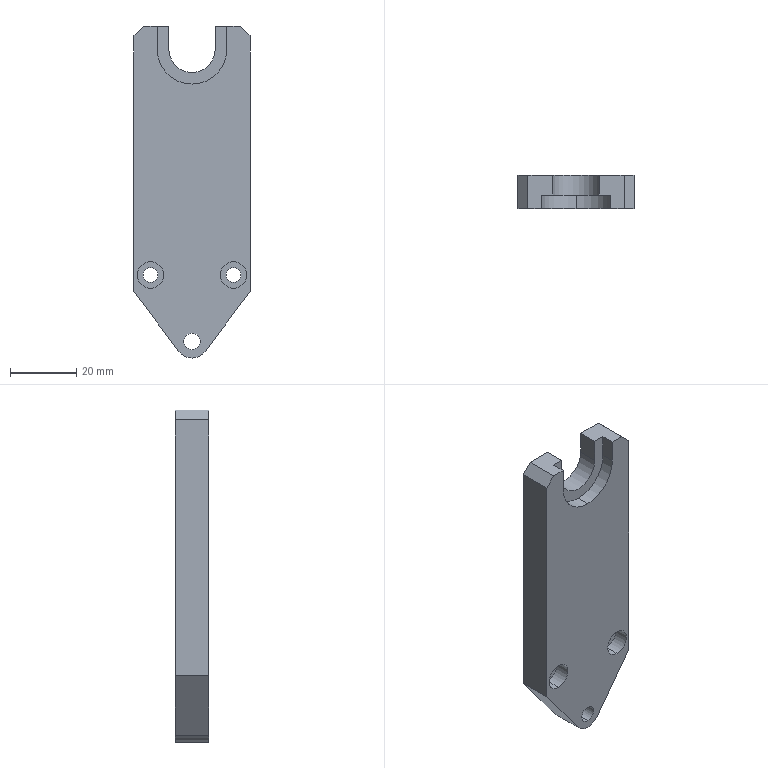Part | SolidWorks | features BaseBody 1 | 1 solid | 32 faces | box 35 x 10 x 100 mm | volume 28731 mm3 | plane 17 | cylinder 15 | commonest cylinder face diameters 4.5 x4 8 x4 5 x2 10 x2 21 x2 14 x1
STEP:
#1=CARTESIAN_POINT('',(0.,5.,-52.5));
#2=VERTEX_POINT('',#1);
#3=CARTESIAN_POINT('',(0.,-5.,-52.5));
#4=VERTEX_POINT('',#3);
#5=CARTESIAN_POINT('',(0.,-5.,-52.5));
#6=DIRECTION('',(0.,-1.,0.));
#7=VECTOR('',#6,1000.);
#8=LINE('',#5,#7);
#9=EDGE_CURVE('',#2,#4,#8,.T.);
#10=ORIENTED_EDGE('',*,*,#9,.F.);
#11=CARTESIAN_POINT('',(0.,5.,-57.5));
#12=VERTEX_POINT('',#11);
#13=CARTESIAN_POINT('',(0.,5.,-55.));
#14=DIRECTION('',(0.,-1.,0.));
#15=DIRECTION('',(0.,0.,-1.));
#16=AXIS2_PLACEMENT_3D('',#13,#14,#15);
#17=CIRCLE('',#16,2.5);
#18=EDGE_CURVE('',#12,#2,#17,.T.);
#19=ORIENTED_EDGE('',*,*,#18,.F.);
#20=CARTESIAN_POINT('',(0.,-5.,-57.5));
#21=VERTEX_POINT('',#20);
#22=CARTESIAN_POINT('',(0.,-5.,-57.5));
#23=DIRECTION('',(0.,-1.,0.));
#24=VECTOR('',#23,1000.);
#25=LINE('',#22,#24);
#26=EDGE_CURVE('',#12,#21,#25,.T.);
#27=ORIENTED_EDGE('',*,*,#26,.T.);
#28=CARTESIAN_POINT('',(0.,-5.,-55.));
#29=DIRECTION('',(0.,-1.,0.));
#30=DIRECTION('',(0.,0.,-1.));
#31=AXIS2_PLACEMENT_3D('',#28,#29,#30);
#32=CIRCLE('',#31,2.5);
#33=EDGE_CURVE('',#21,#4,#32,.T.);
#34=ORIENTED_EDGE('',*,*,#33,.T.);
#35=EDGE_LOOP('',(#10,#19,#27,#34));
#36=FACE_OUTER_BOUND('',#35,.T.);
#37=CARTESIAN_POINT('',(0.,-5.,-55.));
#38=DIRECTION('',(0.,-1.,0.));
#39=DIRECTION('',(0.,0.,-1.));
#40=AXIS2_PLACEMENT_3D('',#37,#38,#39);
#41=CYLINDRICAL_SURFACE('',#40,2.5);
#42=ADVANCED_FACE('',(#36),#41,.F.);
#43=CARTESIAN_POINT('',(-4.,5.,-58.));
#44=VERTEX_POINT('',#43);
#45=CARTESIAN_POINT('',(-17.5,5.,-40.));
#46=VERTEX_POINT('',#45);
#47=CARTESIAN_POINT('',(-17.5,5.,-40.));
#48=DIRECTION('',(-0.6,0.,0.8));
#49=VECTOR('',#48,1000.);
#50=LINE('',#47,#49);
#51=EDGE_CURVE('',#44,#46,#50,.T.);
#52=ORIENTED_EDGE('',*,*,#51,.F.);
#53=CARTESIAN_POINT('',(-4.,-5.,-58.));
#54=VERTEX_POINT('',#53);
#55=CARTESIAN_POINT('',(-4.,45.311,-58.));
#56=DIRECTION('',(0.,-1.,0.));
#57=VECTOR('',#56,1000.);
#58=LINE('',#55,#57);
#59=EDGE_CURVE('',#44,#54,#58,.T.);
#60=ORIENTED_EDGE('',*,*,#59,.T.);
#61=CARTESIAN_POINT('',(-17.5,-5.,-40.));
#62=VERTEX_POINT('',#61);
#63=CARTESIAN_POINT('',(-17.5,-5.,-40.));
#64=DIRECTION('',(0.6,0.,-0.8));
#65=VECTOR('',#64,1000.);
#66=LINE('',#63,#65);
#67=EDGE_CURVE('',#62,#54,#66,.T.);
#68=ORIENTED_EDGE('',*,*,#67,.F.);
#69=CARTESIAN_POINT('',(-17.5,5.,-40.));
#70=DIRECTION('',(0.,-1.,0.));
#71=VECTOR('',#70,1000.);
#72=LINE('',#69,#71);
#73=EDGE_CURVE('',#46,#62,#72,.T.);
#74=ORIENTED_EDGE('',*,*,#73,.F.);
#75=EDGE_LOOP('',(#52,#60,#68,#74));
#76=FACE_OUTER_BOUND('',#75,.T.);
#77=CARTESIAN_POINT('',(-17.5,45.311,-40.));
#78=DIRECTION('',(-0.8,0.,-0.6));
#79=DIRECTION('',(-0.6,0.,0.8));
#80=AXIS2_PLACEMENT_3D('',#77,#78,#79);
#81=PLANE('',#80);
#82=ADVANCED_FACE('',(#76),#81,.T.);
#83=CARTESIAN_POINT('',(0.,5.,-60.));
#84=VERTEX_POINT('',#83);
#85=CARTESIAN_POINT('',(0.,-5.,-60.));
#86=VERTEX_POINT('',#85);
#87=CARTESIAN_POINT('',(0.,45.311,-60.));
#88=DIRECTION('',(0.,-1.,0.));
#89=VECTOR('',#88,1000.);
#90=LINE('',#87,#89);
#91=EDGE_CURVE('',#84,#86,#90,.T.);
#92=ORIENTED_EDGE('',*,*,#91,.F.);
#93=CARTESIAN_POINT('',(4.,5.,-58.));
#94=VERTEX_POINT('',#93);
#95=CARTESIAN_POINT('',(0.,5.,-55.));
#96=DIRECTION('',(0.,1.,0.));
#97=DIRECTION('',(0.,0.,-1.));
#98=AXIS2_PLACEMENT_3D('',#95,#96,#97);
#99=CIRCLE('',#98,5.);
#100=EDGE_CURVE('',#94,#84,#99,.T.);
#101=ORIENTED_EDGE('',*,*,#100,.F.);
#102=CARTESIAN_POINT('',(4.,-5.,-58.));
#103=VERTEX_POINT('',#102);
#104=CARTESIAN_POINT('',(4.,45.311,-58.));
#105=DIRECTION('',(0.,-1.,0.));
#106=VECTOR('',#105,1000.);
#107=LINE('',#104,#106);
#108=EDGE_CURVE('',#94,#103,#107,.T.);
#109=ORIENTED_EDGE('',*,*,#108,.T.);
#110=CARTESIAN_POINT('',(0.,-5.,-55.));
#111=DIRECTION('',(0.,-1.,0.));
#112=DIRECTION('',(0.,0.,-1.));
#113=AXIS2_PLACEMENT_3D('',#110,#111,#112);
#114=CIRCLE('',#113,5.);
#115=EDGE_CURVE('',#86,#103,#114,.T.);
#116=ORIENTED_EDGE('',*,*,#115,.F.);
#117=EDGE_LOOP('',(#92,#101,#109,#116));
#118=FACE_OUTER_BOUND('',#117,.T.);
#119=CARTESIAN_POINT('',(0.,45.311,-55.));
#120=DIRECTION('',(0.,-1.,0.));
#121=DIRECTION('',(0.,0.,-1.));
#122=AXIS2_PLACEMENT_3D('',#119,#120,#121);
#123=CYLINDRICAL_SURFACE('',#122,5.);
#124=ADVANCED_FACE('',(#118),#123,.T.);
#125=CARTESIAN_POINT('',(17.5,5.,-40.));
#126=VERTEX_POINT('',#125);
#127=CARTESIAN_POINT('',(17.5,5.,-40.));
#128=DIRECTION('',(-0.6,0.,-0.8));
#129=VECTOR('',#128,1000.);
#130=LINE('',#127,#129);
#131=EDGE_CURVE('',#126,#94,#130,.T.);
#132=ORIENTED_EDGE('',*,*,#131,.F.);
#133=CARTESIAN_POINT('',(17.5,-5.,-40.));
#134=VERTEX_POINT('',#133);
#135=CARTESIAN_POINT('',(17.5,5.,-40.));
#136=DIRECTION('',(0.,-1.,0.));
#137=VECTOR('',#136,1000.);
#138=LINE('',#135,#137);
#139=EDGE_CURVE('',#126,#134,#138,.T.);
#140=ORIENTED_EDGE('',*,*,#139,.T.);
#141=CARTESIAN_POINT('',(17.5,-5.,-40.));
#142=DIRECTION('',(0.6,0.,0.8));
#143=VECTOR('',#142,1000.);
#144=LINE('',#141,#143);
#145=EDGE_CURVE('',#103,#134,#144,.T.);
#146=ORIENTED_EDGE('',*,*,#145,.F.);
#147=ORIENTED_EDGE('',*,*,#108,.F.);
#148=EDGE_LOOP('',(#132,#140,#146,#147));
#149=FACE_OUTER_BOUND('',#148,.T.);
#150=CARTESIAN_POINT('',(17.5,45.311,-40.));
#151=DIRECTION('',(0.8,0.,-0.6));
#152=DIRECTION('',(0.,-1.,0.));
#153=AXIS2_PLACEMENT_3D('',#150,#151,#152);
#154=PLANE('',#153);
#155=ADVANCED_FACE('',(#149),#154,.T.);
#156=CARTESIAN_POINT('',(12.5,-0.4,-31.));
#157=VERTEX_POINT('',#156);
#158=CARTESIAN_POINT('',(12.5,-5.,-31.));
#159=VERTEX_POINT('',#158);
#160=CARTESIAN_POINT('',(12.5,-5.,-31.));
#161=DIRECTION('',(0.,-1.,0.));
#162=VECTOR('',#161,1000.);
#163=LINE('',#160,#162);
#164=EDGE_CURVE('',#157,#159,#163,.T.);
#165=ORIENTED_EDGE('',*,*,#164,.F.);
#166=CARTESIAN_POINT('',(12.5,-0.4,-39.));
#167=VERTEX_POINT('',#166);
#168=CARTESIAN_POINT('',(12.5,-0.4,-35.));
#169=DIRECTION('',(0.,-1.,0.));
#170=DIRECTION('',(0.,0.,-1.));
#171=AXIS2_PLACEMENT_3D('',#168,#169,#170);
#172=CIRCLE('',#171,4.);
#173=EDGE_CURVE('',#167,#157,#172,.T.);
#174=ORIENTED_EDGE('',*,*,#173,.F.);
#175=CARTESIAN_POINT('',(12.5,-5.,-39.));
#176=VERTEX_POINT('',#175);
#177=CARTESIAN_POINT('',(12.5,-5.,-39.));
#178=DIRECTION('',(0.,-1.,0.));
#179=VECTOR('',#178,1000.);
#180=LINE('',#177,#179);
#181=EDGE_CURVE('',#167,#176,#180,.T.);
#182=ORIENTED_EDGE('',*,*,#181,.T.);
#183=CARTESIAN_POINT('',(12.5,-5.,-35.));
#184=DIRECTION('',(0.,-1.,0.));
#185=DIRECTION('',(0.,0.,-1.));
#186=AXIS2_PLACEMENT_3D('',#183,#184,#185);
#187=CIRCLE('',#186,4.);
#188=EDGE_CURVE('',#176,#159,#187,.T.);
#189=ORIENTED_EDGE('',*,*,#188,.T.);
#190=EDGE_LOOP('',(#165,#174,#182,#189));
#191=FACE_OUTER_BOUND('',#190,.T.);
#192=CARTESIAN_POINT('',(12.5,-5.,-35.));
#193=DIRECTION('',(0.,-1.,0.));
#194=DIRECTION('',(0.,0.,-1.));
#195=AXIS2_PLACEMENT_3D('',#192,#193,#194);
#196=CYLINDRICAL_SURFACE('',#195,4.);
#197=ADVANCED_FACE('',(#191),#196,.F.);
#198=CARTESIAN_POINT('',(12.5,-0.4,-37.25));
#199=VERTEX_POINT('',#198);
#200=CARTESIAN_POINT('',(12.5,-0.4,-32.75));
#201=VERTEX_POINT('',#200);
#202=CARTESIAN_POINT('',(12.5,-0.4,-35.));
#203=DIRECTION('',(0.,-1.,0.));
#204=DIRECTION('',(0.,0.,-1.));
#205=AXIS2_PLACEMENT_3D('',#202,#203,#204);
#206=CIRCLE('',#205,2.25);
#207=EDGE_CURVE('',#199,#201,#206,.T.);
#208=ORIENTED_EDGE('',*,*,#207,.F.);
#209=CARTESIAN_POINT('',(12.5,-0.4,-35.));
#210=DIRECTION('',(0.,-1.,0.));
#211=DIRECTION('',(0.,0.,-1.));
#212=AXIS2_PLACEMENT_3D('',#209,#210,#211);
#213=CIRCLE('',#212,2.25);
#214=EDGE_CURVE('',#201,#199,#213,.T.);
#215=ORIENTED_EDGE('',*,*,#214,.F.);
#216=EDGE_LOOP('',(#208,#215));
#217=FACE_BOUND('',#216,.T.);
#218=ORIENTED_EDGE('',*,*,#173,.T.);
#219=CARTESIAN_POINT('',(12.5,-0.4,-35.));
#220=DIRECTION('',(0.,-1.,0.));
#221=DIRECTION('',(0.,0.,-1.));
#222=AXIS2_PLACEMENT_3D('',#219,#220,#221);
#223=CIRCLE('',#222,4.);
#224=EDGE_CURVE('',#157,#167,#223,.T.);
#225=ORIENTED_EDGE('',*,*,#224,.T.);
#226=EDGE_LOOP('',(#218,#225));
#227=FACE_OUTER_BOUND('',#226,.T.);
#228=CARTESIAN_POINT('',(14.75,-0.4,-35.));
#229=DIRECTION('',(0.,1.,0.));
#230=DIRECTION('',(1.,0.,0.));
#231=AXIS2_PLACEMENT_3D('',#228,#229,#230);
#232=PLANE('',#231);
#233=ADVANCED_FACE('',(#217,#227),#232,.F.);
#234=CARTESIAN_POINT('',(12.5,5.,-32.75));
#235=VERTEX_POINT('',#234);
#236=CARTESIAN_POINT('',(12.5,-5.,-32.75));
#237=DIRECTION('',(0.,-1.,0.));
#238=VECTOR('',#237,1000.);
#239=LINE('',#236,#238);
#240=EDGE_CURVE('',#235,#201,#239,.T.);
#241=ORIENTED_EDGE('',*,*,#240,.F.);
#242=CARTESIAN_POINT('',(12.5,5.,-37.25));
#243=VERTEX_POINT('',#242);
#244=CARTESIAN_POINT('',(12.5,5.,-35.));
#245=DIRECTION('',(0.,-1.,0.));
#246=DIRECTION('',(0.,0.,-1.));
#247=AXIS2_PLACEMENT_3D('',#244,#245,#246);
#248=CIRCLE('',#247,2.25);
#249=EDGE_CURVE('',#243,#235,#248,.T.);
#250=ORIENTED_EDGE('',*,*,#249,.F.);
#251=CARTESIAN_POINT('',(12.5,-5.,-37.25));
#252=DIRECTION('',(0.,-1.,0.));
#253=VECTOR('',#252,1000.);
#254=LINE('',#251,#253);
#255=EDGE_CURVE('',#243,#199,#254,.T.);
#256=ORIENTED_EDGE('',*,*,#255,.T.);
#257=ORIENTED_EDGE('',*,*,#207,.T.);
#258=EDGE_LOOP('',(#241,#250,#256,#257));
#259=FACE_OUTER_BOUND('',#258,.T.);
#260=CARTESIAN_POINT('',(12.5,-5.,-35.));
#261=DIRECTION('',(0.,-1.,0.));
#262=DIRECTION('',(0.,0.,-1.));
#263=AXIS2_PLACEMENT_3D('',#260,#261,#262);
#264=CYLINDRICAL_SURFACE('',#263,2.25);
#265=ADVANCED_FACE('',(#259),#264,.F.);
#266=CARTESIAN_POINT('',(-12.5,-0.4,-31.));
#267=VERTEX_POINT('',#266);
#268=CARTESIAN_POINT('',(-12.5,-5.,-31.));
#269=VERTEX_POINT('',#268);
#270=CARTESIAN_POINT('',(-12.5,-5.,-31.));
#271=DIRECTION('',(0.,-1.,0.));
#272=VECTOR('',#271,1000.);
#273=LINE('',#270,#272);
#274=EDGE_CURVE('',#267,#269,#273,.T.);
#275=ORIENTED_EDGE('',*,*,#274,.F.);
#276=CARTESIAN_POINT('',(-12.5,-0.4,-39.));
#277=VERTEX_POINT('',#276);
#278=CARTESIAN_POINT('',(-12.5,-0.4,-35.));
#279=DIRECTION('',(0.,-1.,0.));
#280=DIRECTION('',(0.,0.,-1.));
#281=AXIS2_PLACEMENT_3D('',#278,#279,#280);
#282=CIRCLE('',#281,4.);
#283=EDGE_CURVE('',#277,#267,#282,.T.);
#284=ORIENTED_EDGE('',*,*,#283,.F.);
#285=CARTESIAN_POINT('',(-12.5,-5.,-39.));
#286=VERTEX_POINT('',#285);
#287=CARTESIAN_POINT('',(-12.5,-5.,-39.));
#288=DIRECTION('',(0.,-1.,0.));
#289=VECTOR('',#288,1000.);
#290=LINE('',#287,#289);
#291=EDGE_CURVE('',#277,#286,#290,.T.);
#292=ORIENTED_EDGE('',*,*,#291,.T.);
#293=CARTESIAN_POINT('',(-12.5,-5.,-35.));
#294=DIRECTION('',(0.,-1.,0.));
#295=DIRECTION('',(0.,0.,-1.));
#296=AXIS2_PLACEMENT_3D('',#293,#294,#295);
#297=CIRCLE('',#296,4.);
#298=EDGE_CURVE('',#286,#269,#297,.T.);
#299=ORIENTED_EDGE('',*,*,#298,.T.);
#300=EDGE_LOOP('',(#275,#284,#292,#299));
#301=FACE_OUTER_BOUND('',#300,.T.);
#302=CARTESIAN_POINT('',(-12.5,-5.,-35.));
#303=DIRECTION('',(0.,-1.,0.));
#304=DIRECTION('',(0.,0.,-1.));
#305=AXIS2_PLACEMENT_3D('',#302,#303,#304);
#306=CYLINDRICAL_SURFACE('',#305,4.);
#307=ADVANCED_FACE('',(#301),#306,.F.);
#308=CARTESIAN_POINT('',(-12.5,-0.4,-37.25));
#309=VERTEX_POINT('',#308);
#310=CARTESIAN_POINT('',(-12.5,-0.4,-32.75));
#311=VERTEX_POINT('',#310);
#312=CARTESIAN_POINT('',(-12.5,-0.4,-35.));
#313=DIRECTION('',(0.,-1.,0.));
#314=DIRECTION('',(0.,0.,-1.));
#315=AXIS2_PLACEMENT_3D('',#312,#313,#314);
#316=CIRCLE('',#315,2.25);
#317=EDGE_CURVE('',#309,#311,#316,.T.);
#318=ORIENTED_EDGE('',*,*,#317,.F.);
#319=CARTESIAN_POINT('',(-12.5,-0.4,-35.));
#320=DIRECTION('',(0.,-1.,0.));
#321=DIRECTION('',(0.,0.,-1.));
#322=AXIS2_PLACEMENT_3D('',#319,#320,#321);
#323=CIRCLE('',#322,2.25);
#324=EDGE_CURVE('',#311,#309,#323,.T.);
#325=ORIENTED_EDGE('',*,*,#324,.F.);
#326=EDGE_LOOP('',(#318,#325));
#327=FACE_BOUND('',#326,.T.);
#328=ORIENTED_EDGE('',*,*,#283,.T.);
#329=CARTESIAN_POINT('',(-12.5,-0.4,-35.));
#330=DIRECTION('',(0.,-1.,0.));
#331=DIRECTION('',(0.,0.,-1.));
#332=AXIS2_PLACEMENT_3D('',#329,#330,#331);
#333=CIRCLE('',#332,4.);
#334=EDGE_CURVE('',#267,#277,#333,.T.);
#335=ORIENTED_EDGE('',*,*,#334,.T.);
#336=EDGE_LOOP('',(#328,#335));
#337=FACE_OUTER_BOUND('',#336,.T.);
#338=CARTESIAN_POINT('',(-10.25,-0.4,-35.));
#339=DIRECTION('',(0.,1.,0.));
#340=DIRECTION('',(1.,0.,0.));
#341=AXIS2_PLACEMENT_3D('',#338,#339,#340);
#342=PLANE('',#341);
#343=ADVANCED_FACE('',(#327,#337),#342,.F.);
#344=CARTESIAN_POINT('',(-12.5,5.,-32.75));
#345=VERTEX_POINT('',#344);
#346=CARTESIAN_POINT('',(-12.5,-5.,-32.75));
#347=DIRECTION('',(0.,-1.,0.));
#348=VECTOR('',#347,1000.);
#349=LINE('',#346,#348);
#350=EDGE_CURVE('',#345,#311,#349,.T.);
#351=ORIENTED_EDGE('',*,*,#350,.F.);
#352=CARTESIAN_POINT('',(-12.5,5.,-37.25));
#353=VERTEX_POINT('',#352);
#354=CARTESIAN_POINT('',(-12.5,5.,-35.));
#355=DIRECTION('',(0.,-1.,0.));
#356=DIRECTION('',(0.,0.,-1.));
#357=AXIS2_PLACEMENT_3D('',#354,#355,#356);
#358=CIRCLE('',#357,2.25);
#359=EDGE_CURVE('',#353,#345,#358,.T.);
#360=ORIENTED_EDGE('',*,*,#359,.F.);
#361=CARTESIAN_POINT('',(-12.5,-5.,-37.25));
#362=DIRECTION('',(0.,-1.,0.));
#363=VECTOR('',#362,1000.);
#364=LINE('',#361,#363);
#365=EDGE_CURVE('',#353,#309,#364,.T.);
#366=ORIENTED_EDGE('',*,*,#365,.T.);
#367=ORIENTED_EDGE('',*,*,#317,.T.);
#368=EDGE_LOOP('',(#351,#360,#366,#367));
#369=FACE_OUTER_BOUND('',#368,.T.);
#370=CARTESIAN_POINT('',(-12.5,-5.,-35.));
#371=DIRECTION('',(0.,-1.,0.));
#372=DIRECTION('',(0.,0.,-1.));
#373=AXIS2_PLACEMENT_3D('',#370,#371,#372);
#374=CYLINDRICAL_SURFACE('',#373,2.25);
#375=ADVANCED_FACE('',(#369),#374,.F.);
#376=CARTESIAN_POINT('',(-17.5,5.,37.));
#377=VERTEX_POINT('',#376);
#378=CARTESIAN_POINT('',(-14.5,5.,40.));
#379=VERTEX_POINT('',#378);
#380=CARTESIAN_POINT('',(-14.5,5.,40.));
#381=DIRECTION('',(0.7071,0.,0.7071));
#382=VECTOR('',#381,1000.);
#383=LINE('',#380,#382);
#384=EDGE_CURVE('',#377,#379,#383,.T.);
#385=ORIENTED_EDGE('',*,*,#384,.F.);
#386=CARTESIAN_POINT('',(-17.5,-5.,37.));
#387=VERTEX_POINT('',#386);
#388=CARTESIAN_POINT('',(-17.5,5.,37.));
#389=DIRECTION('',(0.,1.,0.));
#390=VECTOR('',#389,1000.);
#391=LINE('',#388,#390);
#392=EDGE_CURVE('',#387,#377,#391,.T.);
#393=ORIENTED_EDGE('',*,*,#392,.F.);
#394=CARTESIAN_POINT('',(-14.5,-5.,40.));
#395=VERTEX_POINT('',#394);
#396=CARTESIAN_POINT('',(-27.25,-5.,27.25));
#397=DIRECTION('',(-0.7071,0.,-0.7071));
#398=VECTOR('',#397,1000.);
#399=LINE('',#396,#398);
#400=EDGE_CURVE('',#395,#387,#399,.T.);
#401=ORIENTED_EDGE('',*,*,#400,.F.);
#402=CARTESIAN_POINT('',(-14.5,5.,40.));
#403=DIRECTION('',(0.,-1.,0.));
#404=VECTOR('',#403,1000.);
#405=LINE('',#402,#404);
#406=EDGE_CURVE('',#379,#395,#405,.T.);
#407=ORIENTED_EDGE('',*,*,#406,.F.);
#408=EDGE_LOOP('',(#385,#393,#401,#407));
#409=FACE_OUTER_BOUND('',#408,.T.);
#410=CARTESIAN_POINT('',(-14.5,5.,40.));
#411=DIRECTION('',(0.7071,0.,-0.7071));
#412=DIRECTION('',(0.,-1.,0.));
#413=AXIS2_PLACEMENT_3D('',#410,#411,#412);
#414=PLANE('',#413);
#415=ADVANCED_FACE('',(#409),#414,.F.);
#416=CARTESIAN_POINT('',(14.5,5.,40.));
#417=VERTEX_POINT('',#416);
#418=CARTESIAN_POINT('',(17.5,5.,37.));
#419=VERTEX_POINT('',#418);
#420=CARTESIAN_POINT('',(17.5,5.,37.));
#421=DIRECTION('',(0.7071,0.,-0.7071));
#422=VECTOR('',#421,1000.);
#423=LINE('',#420,#422);
#424=EDGE_CURVE('',#417,#419,#423,.T.);
#425=ORIENTED_EDGE('',*,*,#424,.F.);
#426=CARTESIAN_POINT('',(14.5,-5.,40.));
#427=VERTEX_POINT('',#426);
#428=CARTESIAN_POINT('',(14.5,5.,40.));
#429=DIRECTION('',(0.,1.,0.));
#430=VECTOR('',#429,1000.);
#431=LINE('',#428,#430);
#432=EDGE_CURVE('',#427,#417,#431,.T.);
#433=ORIENTED_EDGE('',*,*,#432,.F.);
#434=CARTESIAN_POINT('',(17.5,-5.,37.));
#435=VERTEX_POINT('',#434);
#436=CARTESIAN_POINT('',(27.25,-5.,27.25));
#437=DIRECTION('',(-0.7071,0.,0.7071));
#438=VECTOR('',#437,1000.);
#439=LINE('',#436,#438);
#440=EDGE_CURVE('',#435,#427,#439,.T.);
#441=ORIENTED_EDGE('',*,*,#440,.F.);
#442=CARTESIAN_POINT('',(17.5,5.,37.));
#443=DIRECTION('',(0.,-1.,0.));
#444=VECTOR('',#443,1000.);
#445=LINE('',#442,#444);
#446=EDGE_CURVE('',#419,#435,#445,.T.);
#447=ORIENTED_EDGE('',*,*,#446,.F.);
#448=EDGE_LOOP('',(#425,#433,#441,#447));
#449=FACE_OUTER_BOUND('',#448,.T.);
#450=CARTESIAN_POINT('',(17.5,5.,37.));
#451=DIRECTION('',(-0.7071,0.,-0.7071));
#452=DIRECTION('',(-0.7071,0.,0.7071));
#453=AXIS2_PLACEMENT_3D('',#450,#451,#452);
#454=PLANE('',#453);
#455=ADVANCED_FACE('',(#449),#454,.F.);
#456=CARTESIAN_POINT('',(10.5,-5.,33.));
#457=VERTEX_POINT('',#456);
#458=CARTESIAN_POINT('',(10.5,-5.,40.));
#459=VERTEX_POINT('',#458);
#460=CARTESIAN_POINT('',(10.5,-5.,33.));
#461=DIRECTION('',(0.,0.,1.));
#462=VECTOR('',#461,1000.);
#463=LINE('',#460,#462);
#464=EDGE_CURVE('',#457,#459,#463,.T.);
#465=ORIENTED_EDGE('',*,*,#464,.T.);
#466=CARTESIAN_POINT('',(10.5,-1.,40.));
#467=VERTEX_POINT('',#466);
#468=CARTESIAN_POINT('',(10.5,-1.,40.));
#469=DIRECTION('',(0.,-1.,0.));
#470=VECTOR('',#469,1000.);
#471=LINE('',#468,#470);
#472=EDGE_CURVE('',#467,#459,#471,.T.);
#473=ORIENTED_EDGE('',*,*,#472,.F.);
#474=CARTESIAN_POINT('',(10.5,-1.,33.));
#475=VERTEX_POINT('',#474);
#476=CARTESIAN_POINT('',(10.5,-1.,33.));
#477=DIRECTION('',(0.,0.,1.));
#478=VECTOR('',#477,1000.);
#479=LINE('',#476,#478);
#480=EDGE_CURVE('',#475,#467,#479,.T.);
#481=ORIENTED_EDGE('',*,*,#480,.F.);
#482=CARTESIAN_POINT('',(10.5,-1.,33.));
#483=DIRECTION('',(0.,-1.,0.));
#484=VECTOR('',#483,1000.);
#485=LINE('',#482,#484);
#486=EDGE_CURVE('',#475,#457,#485,.T.);
#487=ORIENTED_EDGE('',*,*,#486,.T.);
#488=EDGE_LOOP('',(#465,#473,#481,#487));
#489=FACE_OUTER_BOUND('',#488,.T.);
#490=CARTESIAN_POINT('',(10.5,-1.,33.));
#491=DIRECTION('',(1.,0.,0.));
#492=DIRECTION('',(0.,1.,0.));
#493=AXIS2_PLACEMENT_3D('',#490,#491,#492);
#494=PLANE('',#493);
#495=ADVANCED_FACE('',(#489),#494,.F.);
#496=CARTESIAN_POINT('',(-10.5,-5.,40.));
#497=VERTEX_POINT('',#496);
#498=CARTESIAN_POINT('',(-10.5,-5.,33.));
#499=VERTEX_POINT('',#498);
#500=CARTESIAN_POINT('',(-10.5,-5.,33.));
#501=DIRECTION('',(0.,0.,-1.));
#502=VECTOR('',#501,1000.);
#503=LINE('',#500,#502);
#504=EDGE_CURVE('',#497,#499,#503,.T.);
#505=ORIENTED_EDGE('',*,*,#504,.T.);
#506=CARTESIAN_POINT('',(-10.5,-1.,33.));
#507=VERTEX_POINT('',#506);
#508=CARTESIAN_POINT('',(-10.5,-1.,33.));
#509=DIRECTION('',(0.,-1.,0.));
#510=VECTOR('',#509,1000.);
#511=LINE('',#508,#510);
#512=EDGE_CURVE('',#507,#499,#511,.T.);
#513=ORIENTED_EDGE('',*,*,#512,.F.);
#514=CARTESIAN_POINT('',(-10.5,-1.,40.));
#515=VERTEX_POINT('',#514);
#516=CARTESIAN_POINT('',(-10.5,-1.,33.));
#517=DIRECTION('',(0.,0.,-1.));
#518=VECTOR('',#517,1000.);
#519=LINE('',#516,#518);
#520=EDGE_CURVE('',#515,#507,#519,.T.);
#521=ORIENTED_EDGE('',*,*,#520,.F.);
#522=CARTESIAN_POINT('',(-10.5,-1.,40.));
#523=DIRECTION('',(0.,-1.,0.));
#524=VECTOR('',#523,1000.);
#525=LINE('',#522,#524);
#526=EDGE_CURVE('',#515,#497,#525,.T.);
#527=ORIENTED_EDGE('',*,*,#526,.T.);
#528=EDGE_LOOP('',(#505,#513,#521,#527));
#529=FACE_OUTER_BOUND('',#528,.T.);
#530=CARTESIAN_POINT('',(-10.5,-1.,33.));
#531=DIRECTION('',(-1.,0.,0.));
#532=DIRECTION('',(0.,0.,1.));
#533=AXIS2_PLACEMENT_3D('',#530,#531,#532);
#534=PLANE('',#533);
#535=ADVANCED_FACE('',(#529),#534,.F.);
#536=CARTESIAN_POINT('',(0.,-1.,22.5));
#537=VERTEX_POINT('',#536);
#538=CARTESIAN_POINT('',(0.,-5.,22.5));
#539=VERTEX_POINT('',#538);
#540=CARTESIAN_POINT('',(0.,-1.,22.5));
#541=DIRECTION('',(0.,-1.,0.));
#542=VECTOR('',#541,1000.);
#543=LINE('',#540,#542);
#544=EDGE_CURVE('',#537,#539,#543,.T.);
#545=ORIENTED_EDGE('',*,*,#544,.F.);
#546=CARTESIAN_POINT('',(0.,-1.,33.));
#547=DIRECTION('',(0.,-1.,0.));
#548=DIRECTION('',(0.,0.,-1.));
#549=AXIS2_PLACEMENT_3D('',#546,#547,#548);
#550=CIRCLE('',#549,10.5);
#551=EDGE_CURVE('',#507,#537,#550,.T.);
#552=ORIENTED_EDGE('',*,*,#551,.F.);
#553=ORIENTED_EDGE('',*,*,#512,.T.);
#554=CARTESIAN_POINT('',(0.,-5.,33.));
#555=DIRECTION('',(0.,-1.,0.));
#556=DIRECTION('',(0.,0.,-1.));
#557=AXIS2_PLACEMENT_3D('',#554,#555,#556);
#558=CIRCLE('',#557,10.5);
#559=EDGE_CURVE('',#499,#539,#558,.T.);
#560=ORIENTED_EDGE('',*,*,#559,.T.);
#561=EDGE_LOOP('',(#545,#552,#553,#560));
#562=FACE_OUTER_BOUND('',#561,.T.);
#563=CARTESIAN_POINT('',(0.,-1.,33.));
#564=DIRECTION('',(0.,-1.,0.));
#565=DIRECTION('',(0.,0.,-1.));
#566=AXIS2_PLACEMENT_3D('',#563,#564,#565);
#567=CYLINDRICAL_SURFACE('',#566,10.5);
#568=ADVANCED_FACE('',(#562),#567,.F.);
#569=CARTESIAN_POINT('',(-7.,-1.,40.));
#570=VERTEX_POINT('',#569);
#571=CARTESIAN_POINT('',(-17.5,-1.,40.));
#572=DIRECTION('',(-1.,0.,0.));
#573=VECTOR('',#572,1000.);
#574=LINE('',#571,#573);
#575=EDGE_CURVE('',#570,#515,#574,.T.);
#576=ORIENTED_EDGE('',*,*,#575,.T.);
#577=ORIENTED_EDGE('',*,*,#520,.T.);
#578=ORIENTED_EDGE('',*,*,#551,.T.);
#579=CARTESIAN_POINT('',(0.,-1.,33.));
#580=DIRECTION('',(0.,-1.,0.));
#581=DIRECTION('',(0.,0.,-1.));
#582=AXIS2_PLACEMENT_3D('',#579,#580,#581);
#583=CIRCLE('',#582,10.5);
#584=EDGE_CURVE('',#537,#475,#583,.T.);
#585=ORIENTED_EDGE('',*,*,#584,.T.);
#586=ORIENTED_EDGE('',*,*,#480,.T.);
#587=CARTESIAN_POINT('',(7.,-1.,40.));
#588=VERTEX_POINT('',#587);
#589=CARTESIAN_POINT('',(-17.5,-1.,40.));
#590=DIRECTION('',(-1.,0.,0.));
#591=VECTOR('',#590,1000.);
#592=LINE('',#589,#591);
#593=EDGE_CURVE('',#467,#588,#592,.T.);
#594=ORIENTED_EDGE('',*,*,#593,.T.);
#595=CARTESIAN_POINT('',(7.,-1.,33.));
#596=VERTEX_POINT('',#595);
#597=CARTESIAN_POINT('',(7.,-1.,40.));
#598=DIRECTION('',(0.,0.,-1.));
#599=VECTOR('',#598,1000.);
#600=LINE('',#597,#599);
#601=EDGE_CURVE('',#588,#596,#600,.T.);
#602=ORIENTED_EDGE('',*,*,#601,.T.);
#603=CARTESIAN_POINT('',(-7.,-1.,33.));
#604=VERTEX_POINT('',#603);
#605=CARTESIAN_POINT('',(0.,-1.,33.));
#606=DIRECTION('',(0.,1.,0.));
#607=DIRECTION('',(0.,0.,-1.));
#608=AXIS2_PLACEMENT_3D('',#605,#606,#607);
#609=CIRCLE('',#608,7.);
#610=EDGE_CURVE('',#596,#604,#609,.T.);
#611=ORIENTED_EDGE('',*,*,#610,.T.);
#612=CARTESIAN_POINT('',(-7.,-1.,40.));
#613=DIRECTION('',(0.,0.,1.));
#614=VECTOR('',#613,1000.);
#615=LINE('',#612,#614);
#616=EDGE_CURVE('',#604,#570,#615,.T.);
#617=ORIENTED_EDGE('',*,*,#616,.T.);
#618=EDGE_LOOP('',(#576,#577,#578,#585,#586,#594,#602,#611,#617));
#619=FACE_OUTER_BOUND('',#618,.T.);
#620=CARTESIAN_POINT('',(0.,-1.,33.));
#621=DIRECTION('',(0.,-1.,0.));
#622=DIRECTION('',(0.,0.,-1.));
#623=AXIS2_PLACEMENT_3D('',#620,#621,#622);
#624=PLANE('',#623);
#625=ADVANCED_FACE('',(#619),#624,.T.);
#626=ORIENTED_EDGE('',*,*,#298,.F.);
#627=CARTESIAN_POINT('',(-12.5,-5.,-35.));
#628=DIRECTION('',(0.,-1.,0.));
#629=DIRECTION('',(0.,0.,-1.));
#630=AXIS2_PLACEMENT_3D('',#627,#628,#629);
#631=CIRCLE('',#630,4.);
#632=EDGE_CURVE('',#269,#286,#631,.T.);
#633=ORIENTED_EDGE('',*,*,#632,.F.);
#634=EDGE_LOOP('',(#626,#633));
#635=FACE_BOUND('',#634,.T.);
#636=ORIENTED_EDGE('',*,*,#188,.F.);
#637=CARTESIAN_POINT('',(12.5,-5.,-35.));
#638=DIRECTION('',(0.,-1.,0.));
#639=DIRECTION('',(0.,0.,-1.));
#640=AXIS2_PLACEMENT_3D('',#637,#638,#639);
#641=CIRCLE('',#640,4.);
#642=EDGE_CURVE('',#159,#176,#641,.T.);
#643=ORIENTED_EDGE('',*,*,#642,.F.);
#644=EDGE_LOOP('',(#636,#643));
#645=FACE_BOUND('',#644,.T.);
#646=ORIENTED_EDGE('',*,*,#33,.F.);
#647=CARTESIAN_POINT('',(0.,-5.,-55.));
#648=DIRECTION('',(0.,-1.,0.));
#649=DIRECTION('',(0.,0.,-1.));
#650=AXIS2_PLACEMENT_3D('',#647,#648,#649);
#651=CIRCLE('',#650,2.5);
#652=EDGE_CURVE('',#4,#21,#651,.T.);
#653=ORIENTED_EDGE('',*,*,#652,.F.);
#654=EDGE_LOOP('',(#646,#653));
#655=FACE_BOUND('',#654,.T.);
#656=CARTESIAN_POINT('',(17.5,-5.,40.));
#657=DIRECTION('',(0.,0.,-1.));
#658=VECTOR('',#657,1000.);
#659=LINE('',#656,#658);
#660=EDGE_CURVE('',#435,#134,#659,.T.);
#661=ORIENTED_EDGE('',*,*,#660,.F.);
#662=ORIENTED_EDGE('',*,*,#440,.T.);
#663=CARTESIAN_POINT('',(-17.5,-5.,40.));
#664=DIRECTION('',(1.,0.,0.));
#665=VECTOR('',#664,1000.);
#666=LINE('',#663,#665);
#667=EDGE_CURVE('',#459,#427,#666,.T.);
#668=ORIENTED_EDGE('',*,*,#667,.F.);
#669=ORIENTED_EDGE('',*,*,#464,.F.);
#670=CARTESIAN_POINT('',(0.,-5.,33.));
#671=DIRECTION('',(0.,-1.,0.));
#672=DIRECTION('',(0.,0.,-1.));
#673=AXIS2_PLACEMENT_3D('',#670,#671,#672);
#674=CIRCLE('',#673,10.5);
#675=EDGE_CURVE('',#539,#457,#674,.T.);
#676=ORIENTED_EDGE('',*,*,#675,.F.);
#677=ORIENTED_EDGE('',*,*,#559,.F.);
#678=ORIENTED_EDGE('',*,*,#504,.F.);
#679=CARTESIAN_POINT('',(-17.5,-5.,40.));
#680=DIRECTION('',(1.,0.,0.));
#681=VECTOR('',#680,1000.);
#682=LINE('',#679,#681);
#683=EDGE_CURVE('',#395,#497,#682,.T.);
#684=ORIENTED_EDGE('',*,*,#683,.F.);
#685=ORIENTED_EDGE('',*,*,#400,.T.);
#686=CARTESIAN_POINT('',(-17.5,-5.,40.));
#687=DIRECTION('',(0.,0.,1.));
#688=VECTOR('',#687,1000.);
#689=LINE('',#686,#688);
#690=EDGE_CURVE('',#62,#387,#689,.T.);
#691=ORIENTED_EDGE('',*,*,#690,.F.);
#692=ORIENTED_EDGE('',*,*,#67,.T.);
#693=CARTESIAN_POINT('',(0.,-5.,-55.));
#694=DIRECTION('',(0.,-1.,0.));
#695=DIRECTION('',(0.,0.,-1.));
#696=AXIS2_PLACEMENT_3D('',#693,#694,#695);
#697=CIRCLE('',#696,5.);
#698=EDGE_CURVE('',#54,#86,#697,.T.);
#699=ORIENTED_EDGE('',*,*,#698,.T.);
#700=ORIENTED_EDGE('',*,*,#115,.T.);
#701=ORIENTED_EDGE('',*,*,#145,.T.);
#702=EDGE_LOOP('',(#661,#662,#668,#669,#676,#677,#678,#684,#685,#691,#692,#699,#700,#701));
#703=FACE_OUTER_BOUND('',#702,.T.);
#704=CARTESIAN_POINT('',(0.,-5.,0.));
#705=DIRECTION('',(0.,-1.,0.));
#706=DIRECTION('',(0.,0.,-1.));
#707=AXIS2_PLACEMENT_3D('',#704,#705,#706);
#708=PLANE('',#707);
#709=ADVANCED_FACE('',(#635,#645,#655,#703),#708,.T.);
#710=ORIENTED_EDGE('',*,*,#359,.T.);
#711=CARTESIAN_POINT('',(-12.5,5.,-35.));
#712=DIRECTION('',(0.,-1.,0.));
#713=DIRECTION('',(0.,0.,-1.));
#714=AXIS2_PLACEMENT_3D('',#711,#712,#713);
#715=CIRCLE('',#714,2.25);
#716=EDGE_CURVE('',#345,#353,#715,.T.);
#717=ORIENTED_EDGE('',*,*,#716,.T.);
#718=EDGE_LOOP('',(#710,#717));
#719=FACE_BOUND('',#718,.T.);
#720=ORIENTED_EDGE('',*,*,#249,.T.);
#721=CARTESIAN_POINT('',(12.5,5.,-35.));
#722=DIRECTION('',(0.,-1.,0.));
#723=DIRECTION('',(0.,0.,-1.));
#724=AXIS2_PLACEMENT_3D('',#721,#722,#723);
#725=CIRCLE('',#724,2.25);
#726=EDGE_CURVE('',#235,#243,#725,.T.);
#727=ORIENTED_EDGE('',*,*,#726,.T.);
#728=EDGE_LOOP('',(#720,#727));
#729=FACE_BOUND('',#728,.T.);
#730=ORIENTED_EDGE('',*,*,#18,.T.);
#731=CARTESIAN_POINT('',(0.,5.,-55.));
#732=DIRECTION('',(0.,-1.,0.));
#733=DIRECTION('',(0.,0.,-1.));
#734=AXIS2_PLACEMENT_3D('',#731,#732,#733);
#735=CIRCLE('',#734,2.5);
#736=EDGE_CURVE('',#2,#12,#735,.T.);
#737=ORIENTED_EDGE('',*,*,#736,.T.);
#738=EDGE_LOOP('',(#730,#737));
#739=FACE_BOUND('',#738,.T.);
#740=CARTESIAN_POINT('',(7.,5.,40.));
#741=VERTEX_POINT('',#740);
#742=CARTESIAN_POINT('',(-17.5,5.,40.));
#743=DIRECTION('',(1.,0.,0.));
#744=VECTOR('',#743,1000.);
#745=LINE('',#742,#744);
#746=EDGE_CURVE('',#741,#417,#745,.T.);
#747=ORIENTED_EDGE('',*,*,#746,.T.);
#748=ORIENTED_EDGE('',*,*,#424,.T.);
#749=CARTESIAN_POINT('',(17.5,5.,40.));
#750=DIRECTION('',(0.,0.,-1.));
#751=VECTOR('',#750,1000.);
#752=LINE('',#749,#751);
#753=EDGE_CURVE('',#419,#126,#752,.T.);
#754=ORIENTED_EDGE('',*,*,#753,.T.);
#755=ORIENTED_EDGE('',*,*,#131,.T.);
#756=ORIENTED_EDGE('',*,*,#100,.T.);
#757=CARTESIAN_POINT('',(0.,5.,-55.));
#758=DIRECTION('',(0.,1.,0.));
#759=DIRECTION('',(0.,0.,-1.));
#760=AXIS2_PLACEMENT_3D('',#757,#758,#759);
#761=CIRCLE('',#760,5.);
#762=EDGE_CURVE('',#84,#44,#761,.T.);
#763=ORIENTED_EDGE('',*,*,#762,.T.);
#764=ORIENTED_EDGE('',*,*,#51,.T.);
#765=CARTESIAN_POINT('',(-17.5,5.,40.));
#766=DIRECTION('',(0.,0.,1.));
#767=VECTOR('',#766,1000.);
#768=LINE('',#765,#767);
#769=EDGE_CURVE('',#46,#377,#768,.T.);
#770=ORIENTED_EDGE('',*,*,#769,.T.);
#771=ORIENTED_EDGE('',*,*,#384,.T.);
#772=CARTESIAN_POINT('',(-7.,5.,40.));
#773=VERTEX_POINT('',#772);
#774=CARTESIAN_POINT('',(-17.5,5.,40.));
#775=DIRECTION('',(1.,0.,0.));
#776=VECTOR('',#775,1000.);
#777=LINE('',#774,#776);
#778=EDGE_CURVE('',#379,#773,#777,.T.);
#779=ORIENTED_EDGE('',*,*,#778,.T.);
#780=CARTESIAN_POINT('',(-7.,5.,33.));
#781=VERTEX_POINT('',#780);
#782=CARTESIAN_POINT('',(-7.,5.,40.));
#783=DIRECTION('',(0.,0.,1.));
#784=VECTOR('',#783,1000.);
#785=LINE('',#782,#784);
#786=EDGE_CURVE('',#781,#773,#785,.T.);
#787=ORIENTED_EDGE('',*,*,#786,.F.);
#788=CARTESIAN_POINT('',(7.,5.,33.));
#789=VERTEX_POINT('',#788);
#790=CARTESIAN_POINT('',(0.,5.,33.));
#791=DIRECTION('',(0.,1.,0.));
#792=DIRECTION('',(0.,0.,1.));
#793=AXIS2_PLACEMENT_3D('',#790,#791,#792);
#794=CIRCLE('',#793,7.);
#795=EDGE_CURVE('',#789,#781,#794,.T.);
#796=ORIENTED_EDGE('',*,*,#795,.F.);
#797=CARTESIAN_POINT('',(7.,5.,40.));
#798=DIRECTION('',(0.,0.,-1.));
#799=VECTOR('',#798,1000.);
#800=LINE('',#797,#799);
#801=EDGE_CURVE('',#741,#789,#800,.T.);
#802=ORIENTED_EDGE('',*,*,#801,.F.);
#803=EDGE_LOOP('',(#747,#748,#754,#755,#756,#763,#764,#770,#771,#779,#787,#796,#802));
#804=FACE_OUTER_BOUND('',#803,.T.);
#805=CARTESIAN_POINT('',(0.,5.,0.));
#806=DIRECTION('',(0.,-1.,0.));
#807=DIRECTION('',(0.,0.,-1.));
#808=AXIS2_PLACEMENT_3D('',#805,#806,#807);
#809=PLANE('',#808);
#810=ADVANCED_FACE('',(#719,#729,#739,#804),#809,.F.);
#811=ORIENTED_EDGE('',*,*,#667,.T.);
#812=ORIENTED_EDGE('',*,*,#432,.T.);
#813=ORIENTED_EDGE('',*,*,#746,.F.);
#814=CARTESIAN_POINT('',(7.,-30.239,40.));
#815=DIRECTION('',(0.,1.,0.));
#816=VECTOR('',#815,1000.);
#817=LINE('',#814,#816);
#818=EDGE_CURVE('',#588,#741,#817,.T.);
#819=ORIENTED_EDGE('',*,*,#818,.F.);
#820=ORIENTED_EDGE('',*,*,#593,.F.);
#821=ORIENTED_EDGE('',*,*,#472,.T.);
#822=EDGE_LOOP('',(#811,#812,#813,#819,#820,#821));
#823=FACE_OUTER_BOUND('',#822,.T.);
#824=CARTESIAN_POINT('',(-17.5,5.,40.));
#825=DIRECTION('',(0.,0.,-1.));
#826=DIRECTION('',(0.,-1.,0.));
#827=AXIS2_PLACEMENT_3D('',#824,#825,#826);
#828=PLANE('',#827);
#829=ADVANCED_FACE('',(#823),#828,.F.);
#830=ORIENTED_EDGE('',*,*,#690,.T.);
#831=ORIENTED_EDGE('',*,*,#392,.T.);
#832=ORIENTED_EDGE('',*,*,#769,.F.);
#833=ORIENTED_EDGE('',*,*,#73,.T.);
#834=EDGE_LOOP('',(#830,#831,#832,#833));
#835=FACE_OUTER_BOUND('',#834,.T.);
#836=CARTESIAN_POINT('',(-17.5,5.,40.));
#837=DIRECTION('',(1.,0.,0.));
#838=DIRECTION('',(0.,1.,0.));
#839=AXIS2_PLACEMENT_3D('',#836,#837,#838);
#840=PLANE('',#839);
#841=ADVANCED_FACE('',(#835),#840,.F.);
#842=ORIENTED_EDGE('',*,*,#753,.F.);
#843=ORIENTED_EDGE('',*,*,#446,.T.);
#844=ORIENTED_EDGE('',*,*,#660,.T.);
#845=ORIENTED_EDGE('',*,*,#139,.F.);
#846=EDGE_LOOP('',(#842,#843,#844,#845));
#847=FACE_OUTER_BOUND('',#846,.T.);
#848=CARTESIAN_POINT('',(17.5,5.,40.));
#849=DIRECTION('',(-1.,0.,0.));
#850=DIRECTION('',(0.,0.,1.));
#851=AXIS2_PLACEMENT_3D('',#848,#849,#850);
#852=PLANE('',#851);
#853=ADVANCED_FACE('',(#847),#852,.F.);
#854=ORIENTED_EDGE('',*,*,#778,.F.);
#855=ORIENTED_EDGE('',*,*,#406,.T.);
#856=ORIENTED_EDGE('',*,*,#683,.T.);
#857=ORIENTED_EDGE('',*,*,#526,.F.);
#858=ORIENTED_EDGE('',*,*,#575,.F.);
#859=CARTESIAN_POINT('',(-7.,-30.239,40.));
#860=DIRECTION('',(0.,1.,0.));
#861=VECTOR('',#860,1000.);
#862=LINE('',#859,#861);
#863=EDGE_CURVE('',#570,#773,#862,.T.);
#864=ORIENTED_EDGE('',*,*,#863,.T.);
#865=EDGE_LOOP('',(#854,#855,#856,#857,#858,#864));
#866=FACE_OUTER_BOUND('',#865,.T.);
#867=CARTESIAN_POINT('',(-17.5,5.,40.));
#868=DIRECTION('',(0.,0.,-1.));
#869=DIRECTION('',(0.,-1.,0.));
#870=AXIS2_PLACEMENT_3D('',#867,#868,#869);
#871=PLANE('',#870);
#872=ADVANCED_FACE('',(#866),#871,.F.);
#873=ORIENTED_EDGE('',*,*,#616,.F.);
#874=CARTESIAN_POINT('',(-7.,-30.239,33.));
#875=DIRECTION('',(0.,1.,0.));
#876=VECTOR('',#875,1000.);
#877=LINE('',#874,#876);
#878=EDGE_CURVE('',#604,#781,#877,.T.);
#879=ORIENTED_EDGE('',*,*,#878,.T.);
#880=ORIENTED_EDGE('',*,*,#786,.T.);
#881=ORIENTED_EDGE('',*,*,#863,.F.);
#882=EDGE_LOOP('',(#873,#879,#880,#881));
#883=FACE_OUTER_BOUND('',#882,.T.);
#884=CARTESIAN_POINT('',(-7.,-30.239,40.));
#885=DIRECTION('',(-1.,0.,0.));
#886=DIRECTION('',(0.,0.,1.));
#887=AXIS2_PLACEMENT_3D('',#884,#885,#886);
#888=PLANE('',#887);
#889=ADVANCED_FACE('',(#883),#888,.F.);
#890=ORIENTED_EDGE('',*,*,#610,.F.);
#891=CARTESIAN_POINT('',(7.,-30.239,33.));
#892=DIRECTION('',(0.,1.,0.));
#893=VECTOR('',#892,1000.);
#894=LINE('',#891,#893);
#895=EDGE_CURVE('',#596,#789,#894,.T.);
#896=ORIENTED_EDGE('',*,*,#895,.T.);
#897=ORIENTED_EDGE('',*,*,#795,.T.);
#898=ORIENTED_EDGE('',*,*,#878,.F.);
#899=EDGE_LOOP('',(#890,#896,#897,#898));
#900=FACE_OUTER_BOUND('',#899,.T.);
#901=CARTESIAN_POINT('',(0.,-30.239,33.));
#902=DIRECTION('',(0.,1.,0.));
#903=DIRECTION('',(0.,0.,1.));
#904=AXIS2_PLACEMENT_3D('',#901,#902,#903);
#905=CYLINDRICAL_SURFACE('',#904,7.);
#906=ADVANCED_FACE('',(#900),#905,.F.);
#907=ORIENTED_EDGE('',*,*,#601,.F.);
#908=ORIENTED_EDGE('',*,*,#818,.T.);
#909=ORIENTED_EDGE('',*,*,#801,.T.);
#910=ORIENTED_EDGE('',*,*,#895,.F.);
#911=EDGE_LOOP('',(#907,#908,#909,#910));
#912=FACE_OUTER_BOUND('',#911,.T.);
#913=CARTESIAN_POINT('',(7.,-30.239,40.));
#914=DIRECTION('',(1.,0.,0.));
#915=DIRECTION('',(0.,1.,0.));
#916=AXIS2_PLACEMENT_3D('',#913,#914,#915);
#917=PLANE('',#916);
#918=ADVANCED_FACE('',(#912),#917,.F.);
#919=ORIENTED_EDGE('',*,*,#584,.F.);
#920=ORIENTED_EDGE('',*,*,#544,.T.);
#921=ORIENTED_EDGE('',*,*,#675,.T.);
#922=ORIENTED_EDGE('',*,*,#486,.F.);
#923=EDGE_LOOP('',(#919,#920,#921,#922));
#924=FACE_OUTER_BOUND('',#923,.T.);
#925=CARTESIAN_POINT('',(0.,-1.,33.));
#926=DIRECTION('',(0.,-1.,0.));
#927=DIRECTION('',(0.,0.,-1.));
#928=AXIS2_PLACEMENT_3D('',#925,#926,#927);
#929=CYLINDRICAL_SURFACE('',#928,10.5);
#930=ADVANCED_FACE('',(#924),#929,.F.);
#931=ORIENTED_EDGE('',*,*,#716,.F.);
#932=ORIENTED_EDGE('',*,*,#350,.T.);
#933=ORIENTED_EDGE('',*,*,#324,.T.);
#934=ORIENTED_EDGE('',*,*,#365,.F.);
#935=EDGE_LOOP('',(#931,#932,#933,#934));
#936=FACE_OUTER_BOUND('',#935,.T.);
#937=CARTESIAN_POINT('',(-12.5,-5.,-35.));
#938=DIRECTION('',(0.,-1.,0.));
#939=DIRECTION('',(0.,0.,-1.));
#940=AXIS2_PLACEMENT_3D('',#937,#938,#939);
#941=CYLINDRICAL_SURFACE('',#940,2.25);
#942=ADVANCED_FACE('',(#936),#941,.F.);
#943=ORIENTED_EDGE('',*,*,#334,.F.);
#944=ORIENTED_EDGE('',*,*,#274,.T.);
#945=ORIENTED_EDGE('',*,*,#632,.T.);
#946=ORIENTED_EDGE('',*,*,#291,.F.);
#947=EDGE_LOOP('',(#943,#944,#945,#946));
#948=FACE_OUTER_BOUND('',#947,.T.);
#949=CARTESIAN_POINT('',(-12.5,-5.,-35.));
#950=DIRECTION('',(0.,-1.,0.));
#951=DIRECTION('',(0.,0.,-1.));
#952=AXIS2_PLACEMENT_3D('',#949,#950,#951);
#953=CYLINDRICAL_SURFACE('',#952,4.);
#954=ADVANCED_FACE('',(#948),#953,.F.);
#955=ORIENTED_EDGE('',*,*,#726,.F.);
#956=ORIENTED_EDGE('',*,*,#240,.T.);
#957=ORIENTED_EDGE('',*,*,#214,.T.);
#958=ORIENTED_EDGE('',*,*,#255,.F.);
#959=EDGE_LOOP('',(#955,#956,#957,#958));
#960=FACE_OUTER_BOUND('',#959,.T.);
#961=CARTESIAN_POINT('',(12.5,-5.,-35.));
#962=DIRECTION('',(0.,-1.,0.));
#963=DIRECTION('',(0.,0.,-1.));
#964=AXIS2_PLACEMENT_3D('',#961,#962,#963);
#965=CYLINDRICAL_SURFACE('',#964,2.25);
#966=ADVANCED_FACE('',(#960),#965,.F.);
#967=ORIENTED_EDGE('',*,*,#224,.F.);
#968=ORIENTED_EDGE('',*,*,#164,.T.);
#969=ORIENTED_EDGE('',*,*,#642,.T.);
#970=ORIENTED_EDGE('',*,*,#181,.F.);
#971=EDGE_LOOP('',(#967,#968,#969,#970));
#972=FACE_OUTER_BOUND('',#971,.T.);
#973=CARTESIAN_POINT('',(12.5,-5.,-35.));
#974=DIRECTION('',(0.,-1.,0.));
#975=DIRECTION('',(0.,0.,-1.));
#976=AXIS2_PLACEMENT_3D('',#973,#974,#975);
#977=CYLINDRICAL_SURFACE('',#976,4.);
#978=ADVANCED_FACE('',(#972),#977,.F.);
#979=ORIENTED_EDGE('',*,*,#762,.F.);
#980=ORIENTED_EDGE('',*,*,#91,.T.);
#981=ORIENTED_EDGE('',*,*,#698,.F.);
#982=ORIENTED_EDGE('',*,*,#59,.F.);
#983=EDGE_LOOP('',(#979,#980,#981,#982));
#984=FACE_OUTER_BOUND('',#983,.T.);
#985=CARTESIAN_POINT('',(0.,45.311,-55.));
#986=DIRECTION('',(0.,-1.,0.));
#987=DIRECTION('',(0.,0.,-1.));
#988=AXIS2_PLACEMENT_3D('',#985,#986,#987);
#989=CYLINDRICAL_SURFACE('',#988,5.);
#990=ADVANCED_FACE('',(#984),#989,.T.);
#991=ORIENTED_EDGE('',*,*,#736,.F.);
#992=ORIENTED_EDGE('',*,*,#9,.T.);
#993=ORIENTED_EDGE('',*,*,#652,.T.);
#994=ORIENTED_EDGE('',*,*,#26,.F.);
#995=EDGE_LOOP('',(#991,#992,#993,#994));
#996=FACE_OUTER_BOUND('',#995,.T.);
#997=CARTESIAN_POINT('',(0.,-5.,-55.));
#998=DIRECTION('',(0.,-1.,0.));
#999=DIRECTION('',(0.,0.,-1.));
#1000=AXIS2_PLACEMENT_3D('',#997,#998,#999);
#1001=CYLINDRICAL_SURFACE('',#1000,2.5);
#1002=ADVANCED_FACE('',(#996),#1001,.F.);
#1003=CLOSED_SHELL('',(#42,#82,#124,#155,#197,#233,#265,#307,#343,#375,#415,#455,#495,#535,#568,#625,#709,#810,#829,#841,#853,#872,#889,#906,#918,#930,#942,#954,#966,#978,#990,#1002));
#1004=MANIFOLD_SOLID_BREP('',#1003);
#1005=CARTESIAN_POINT('',(0.,0.,0.));
#1006=DIRECTION('',(0.,0.,1.));
#1007=DIRECTION('',(1.,0.,0.));
#1008=AXIS2_PLACEMENT_3D('',#1005,#1006,#1007);
#1009=(LENGTH_UNIT()NAMED_UNIT(*)SI_UNIT(.MILLI.,.METRE.));
#1010=UNCERTAINTY_MEASURE_WITH_UNIT(LENGTH_MEASURE(0.00001),#1009,'','');
#1011=(NAMED_UNIT(*)PLANE_ANGLE_UNIT()SI_UNIT($,.RADIAN.));
#1012=(NAMED_UNIT(*)SI_UNIT($,.STERADIAN.)SOLID_ANGLE_UNIT());
#1013=(GEOMETRIC_REPRESENTATION_CONTEXT(3)GLOBAL_UNCERTAINTY_ASSIGNED_CONTEXT((#1010))GLOBAL_UNIT_ASSIGNED_CONTEXT((#1009,#1011,#1012))REPRESENTATION_CONTEXT('',''));
#1014=ADVANCED_BREP_SHAPE_REPRESENTATION('',(#1004,#1008),#1013);